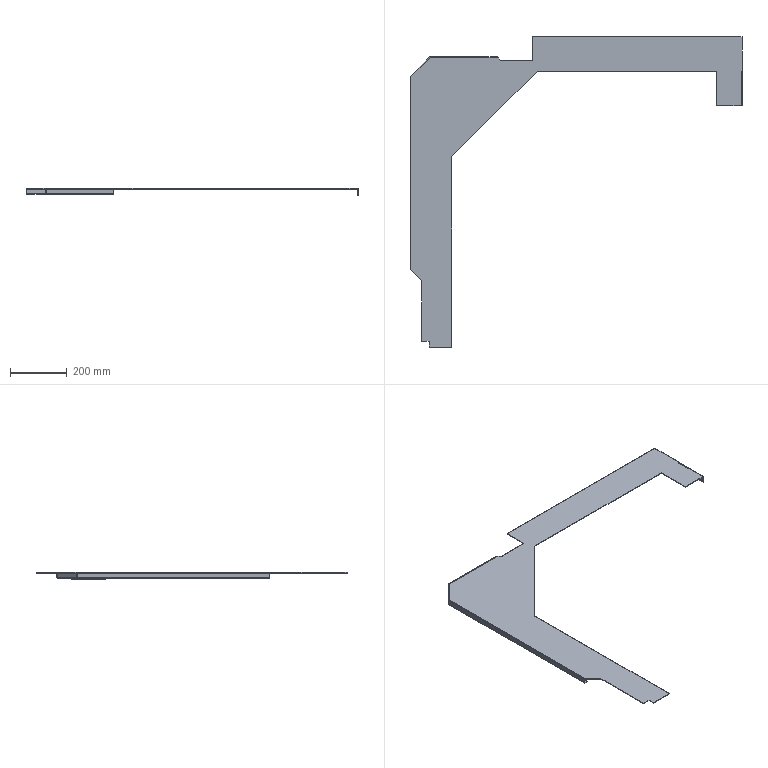Part | STEP file | Center Shaft Plate | 1 solid | 76 faces | box 1167 x 1091 x 25 mm | volume 650871 mm3 | plane 49 | cylinder 19 | spline 8 | commonest cylinder face diameters 1 x7 5 x7 0.4 x4 4 x1